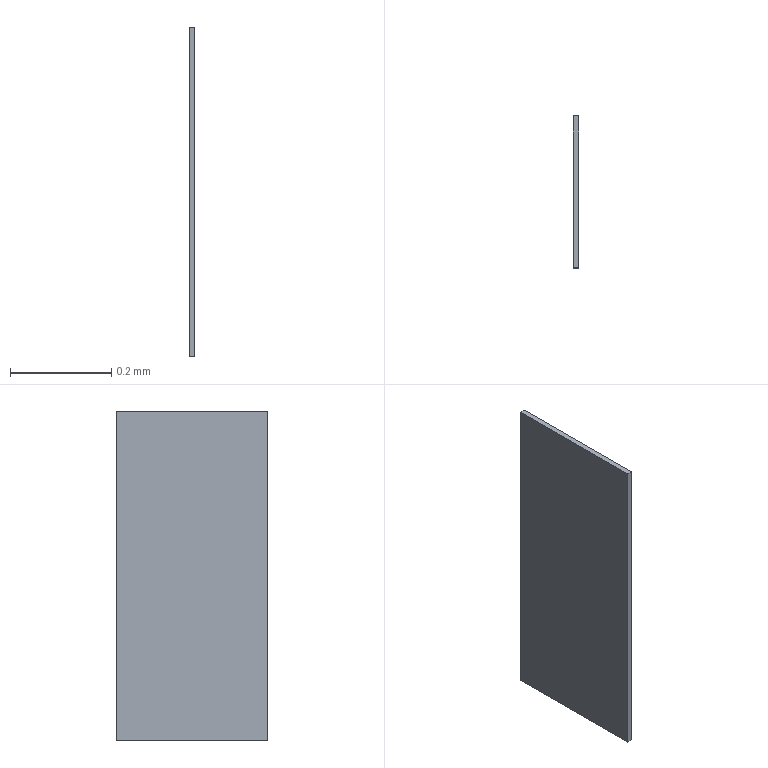Part | Creo | 1 solid | 6 faces | box 0.01 x 0.3 x 0.65 mm | volume 0.00195 mm3 | plane 6
STEP:
#1=CARTESIAN_POINT('',(0.,0.,0.));
#2=DIRECTION('',(0.,0.,1.));
#3=DIRECTION('',(1.,0.,0.));
#4=AXIS2_PLACEMENT_3D('',#1,#2,#3);
#5=CARTESIAN_POINT('',(0.12,-5.25,-1.73));
#6=VERTEX_POINT('',#5);
#7=CARTESIAN_POINT('',(0.12,-5.55,-1.73));
#8=VERTEX_POINT('',#7);
#9=CARTESIAN_POINT('',(0.12,-5.25,-1.73));
#10=DIRECTION('',(0.,-1.,0.));
#11=VECTOR('',#10,0.3);
#12=LINE('',#9,#11);
#13=EDGE_CURVE('',#6,#8,#12,.T.);
#14=ORIENTED_EDGE('',*,*,#13,.T.);
#15=CARTESIAN_POINT('',(0.12,-5.55,-1.08));
#16=VERTEX_POINT('',#15);
#17=CARTESIAN_POINT('',(0.12,-5.55,-1.08));
#18=DIRECTION('',(0.,0.,-1.));
#19=VECTOR('',#18,0.65);
#20=LINE('',#17,#19);
#21=EDGE_CURVE('',#16,#8,#20,.T.);
#22=ORIENTED_EDGE('',*,*,#21,.F.);
#23=CARTESIAN_POINT('',(0.12,-5.25,-1.08));
#24=VERTEX_POINT('',#23);
#25=CARTESIAN_POINT('',(0.12,-5.25,-1.08));
#26=DIRECTION('',(0.,-1.,0.));
#27=VECTOR('',#26,0.3);
#28=LINE('',#25,#27);
#29=EDGE_CURVE('',#24,#16,#28,.T.);
#30=ORIENTED_EDGE('',*,*,#29,.F.);
#31=CARTESIAN_POINT('',(0.12,-5.25,-1.73));
#32=DIRECTION('',(0.,0.,1.));
#33=VECTOR('',#32,0.65);
#34=LINE('',#31,#33);
#35=EDGE_CURVE('',#6,#24,#34,.T.);
#36=ORIENTED_EDGE('',*,*,#35,.F.);
#37=EDGE_LOOP('',(#14,#22,#30,#36));
#38=FACE_OUTER_BOUND('',#37,.F.);
#39=CARTESIAN_POINT('',(0.12,0.,0.));
#40=DIRECTION('',(1.,0.,0.));
#41=DIRECTION('',(0.,-1.,0.));
#42=AXIS2_PLACEMENT_3D('',#39,#40,#41);
#43=PLANE('',#42);
#44=ADVANCED_FACE('',(#38),#43,.T.);
#45=CARTESIAN_POINT('',(0.11,-5.25,-1.73));
#46=VERTEX_POINT('',#45);
#47=CARTESIAN_POINT('',(0.11,-5.55,-1.73));
#48=VERTEX_POINT('',#47);
#49=CARTESIAN_POINT('',(0.11,-5.25,-1.73));
#50=DIRECTION('',(0.,-1.,0.));
#51=VECTOR('',#50,0.3);
#52=LINE('',#49,#51);
#53=EDGE_CURVE('',#46,#48,#52,.T.);
#54=ORIENTED_EDGE('',*,*,#53,.T.);
#55=CARTESIAN_POINT('',(0.11,-5.55,-1.73));
#56=DIRECTION('',(1.,0.,0.));
#57=VECTOR('',#56,0.01);
#58=LINE('',#55,#57);
#59=EDGE_CURVE('',#48,#8,#58,.T.);
#60=ORIENTED_EDGE('',*,*,#59,.T.);
#61=ORIENTED_EDGE('',*,*,#13,.F.);
#62=CARTESIAN_POINT('',(0.11,-5.25,-1.73));
#63=DIRECTION('',(1.,0.,0.));
#64=VECTOR('',#63,0.01);
#65=LINE('',#62,#64);
#66=EDGE_CURVE('',#46,#6,#65,.T.);
#67=ORIENTED_EDGE('',*,*,#66,.F.);
#68=EDGE_LOOP('',(#54,#60,#61,#67));
#69=FACE_OUTER_BOUND('',#68,.F.);
#70=CARTESIAN_POINT('',(0.12,1.35,-1.73));
#71=DIRECTION('',(0.,0.,1.));
#72=DIRECTION('',(0.,-1.,0.));
#73=AXIS2_PLACEMENT_3D('',#70,#71,#72);
#74=PLANE('',#73);
#75=ADVANCED_FACE('',(#69),#74,.F.);
#76=CARTESIAN_POINT('',(0.11,-5.25,-1.08));
#77=VERTEX_POINT('',#76);
#78=CARTESIAN_POINT('',(0.11,-5.25,-1.73));
#79=DIRECTION('',(0.,0.,1.));
#80=VECTOR('',#79,0.65);
#81=LINE('',#78,#80);
#82=EDGE_CURVE('',#46,#77,#81,.T.);
#83=ORIENTED_EDGE('',*,*,#82,.T.);
#84=CARTESIAN_POINT('',(0.11,-5.55,-1.08));
#85=VERTEX_POINT('',#84);
#86=CARTESIAN_POINT('',(0.11,-5.25,-1.08));
#87=DIRECTION('',(0.,-1.,0.));
#88=VECTOR('',#87,0.3);
#89=LINE('',#86,#88);
#90=EDGE_CURVE('',#77,#85,#89,.T.);
#91=ORIENTED_EDGE('',*,*,#90,.T.);
#92=CARTESIAN_POINT('',(0.11,-5.55,-1.08));
#93=DIRECTION('',(0.,0.,-1.));
#94=VECTOR('',#93,0.65);
#95=LINE('',#92,#94);
#96=EDGE_CURVE('',#85,#48,#95,.T.);
#97=ORIENTED_EDGE('',*,*,#96,.T.);
#98=ORIENTED_EDGE('',*,*,#53,.F.);
#99=EDGE_LOOP('',(#83,#91,#97,#98));
#100=FACE_OUTER_BOUND('',#99,.F.);
#101=CARTESIAN_POINT('',(0.11,-11.395,4.186));
#102=DIRECTION('',(1.,0.,0.));
#103=DIRECTION('',(0.,1.,0.));
#104=AXIS2_PLACEMENT_3D('',#101,#102,#103);
#105=PLANE('',#104);
#106=ADVANCED_FACE('',(#100),#105,.F.);
#107=ORIENTED_EDGE('',*,*,#82,.F.);
#108=ORIENTED_EDGE('',*,*,#66,.T.);
#109=ORIENTED_EDGE('',*,*,#35,.T.);
#110=CARTESIAN_POINT('',(0.11,-5.25,-1.08));
#111=DIRECTION('',(1.,0.,0.));
#112=VECTOR('',#111,0.01);
#113=LINE('',#110,#112);
#114=EDGE_CURVE('',#77,#24,#113,.T.);
#115=ORIENTED_EDGE('',*,*,#114,.F.);
#116=EDGE_LOOP('',(#107,#108,#109,#115));
#117=FACE_OUTER_BOUND('',#116,.F.);
#118=CARTESIAN_POINT('',(0.,-5.25,-1.88));
#119=DIRECTION('',(0.,1.,0.));
#120=DIRECTION('',(0.,0.,1.));
#121=AXIS2_PLACEMENT_3D('',#118,#119,#120);
#122=PLANE('',#121);
#123=ADVANCED_FACE('',(#117),#122,.T.);
#124=ORIENTED_EDGE('',*,*,#90,.F.);
#125=ORIENTED_EDGE('',*,*,#114,.T.);
#126=ORIENTED_EDGE('',*,*,#29,.T.);
#127=CARTESIAN_POINT('',(0.11,-5.55,-1.08));
#128=DIRECTION('',(1.,0.,0.));
#129=VECTOR('',#128,0.01);
#130=LINE('',#127,#129);
#131=EDGE_CURVE('',#85,#16,#130,.T.);
#132=ORIENTED_EDGE('',*,*,#131,.F.);
#133=EDGE_LOOP('',(#124,#125,#126,#132));
#134=FACE_OUTER_BOUND('',#133,.F.);
#135=CARTESIAN_POINT('',(0.,-5.25,-1.08));
#136=DIRECTION('',(0.,0.,1.));
#137=DIRECTION('',(0.,-1.,0.));
#138=AXIS2_PLACEMENT_3D('',#135,#136,#137);
#139=PLANE('',#138);
#140=ADVANCED_FACE('',(#134),#139,.T.);
#141=ORIENTED_EDGE('',*,*,#96,.F.);
#142=ORIENTED_EDGE('',*,*,#131,.T.);
#143=ORIENTED_EDGE('',*,*,#21,.T.);
#144=ORIENTED_EDGE('',*,*,#59,.F.);
#145=EDGE_LOOP('',(#141,#142,#143,#144));
#146=FACE_OUTER_BOUND('',#145,.F.);
#147=CARTESIAN_POINT('',(0.,-5.55,-1.08));
#148=DIRECTION('',(0.,-1.,0.));
#149=DIRECTION('',(0.,0.,-1.));
#150=AXIS2_PLACEMENT_3D('',#147,#148,#149);
#151=PLANE('',#150);
#152=ADVANCED_FACE('',(#146),#151,.T.);
#153=CLOSED_SHELL('',(#44,#75,#106,#123,#140,#152));
#154=MANIFOLD_SOLID_BREP('',#153);
#155=(LENGTH_UNIT()NAMED_UNIT(*)SI_UNIT(.MILLI.,.METRE.));
#156=UNCERTAINTY_MEASURE_WITH_UNIT(LENGTH_MEASURE(0.00007159),#155,'','');
#157=(NAMED_UNIT(*)PLANE_ANGLE_UNIT()SI_UNIT($,.RADIAN.));
#158=PLANE_ANGLE_MEASURE_WITH_UNIT(PLANE_ANGLE_MEASURE(0.01745),#157);
#159=(CONVERSION_BASED_UNIT('DEGREE',#158)NAMED_UNIT(*)PLANE_ANGLE_UNIT());
#160=(NAMED_UNIT(*)SI_UNIT($,.STERADIAN.)SOLID_ANGLE_UNIT());
#161=(GEOMETRIC_REPRESENTATION_CONTEXT(3)GLOBAL_UNCERTAINTY_ASSIGNED_CONTEXT((#156))GLOBAL_UNIT_ASSIGNED_CONTEXT((#155,#159,#160))REPRESENTATION_CONTEXT('',''));
#162=ADVANCED_BREP_SHAPE_REPRESENTATION('',(#4,#154),#161);